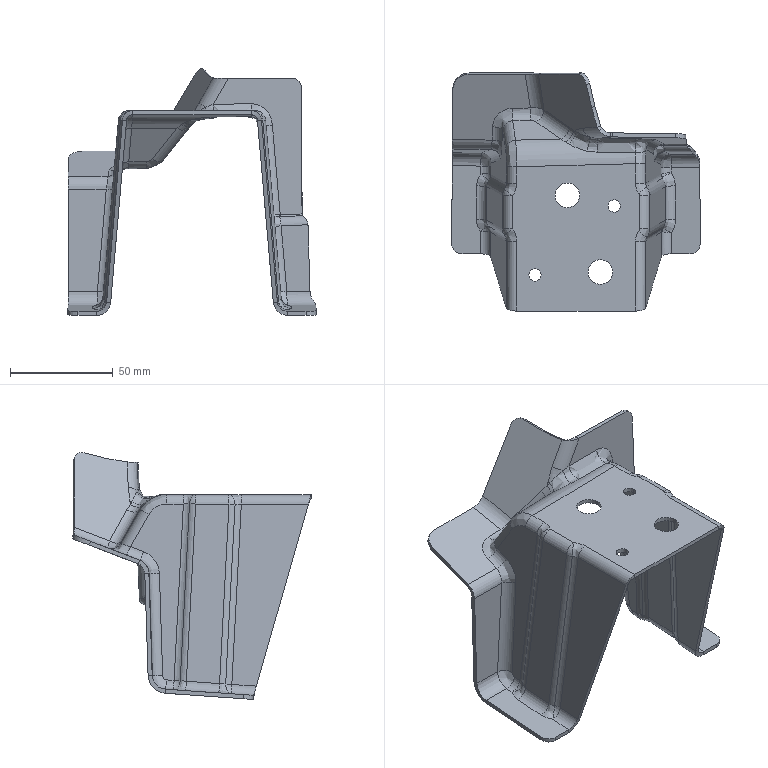Part | 1 solid | 220 faces | box 121.241 x 116.196 x 120.431 mm | volume 53068 mm3 | spline 102 | cylinder 78 | plane 27 | sphere 8 | other 5 | commonest cylinder face diameters 10 x31 14 x21 6 x16 12 x4 18 x2 16 x1